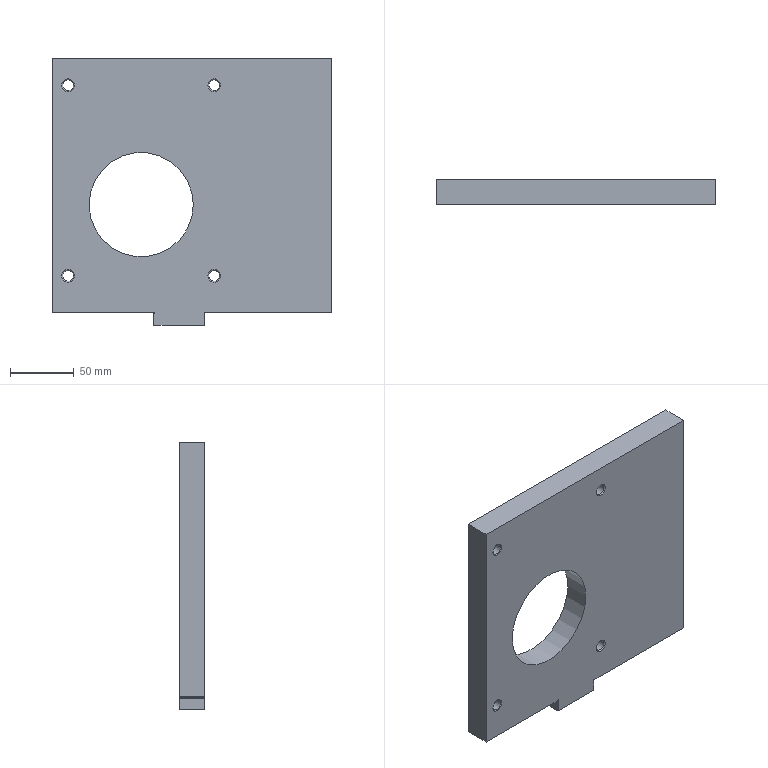Part | STEP file | YBQDJ-YB-18 | 1 solid | 41 faces | box 220 x 20 x 210 mm | volume 773333 mm3 | cone 16 | cylinder 15 | plane 10 | commonest cylinder face diameters 8.5 x6 2 x4 1 x2 6.8 x2 82 x1